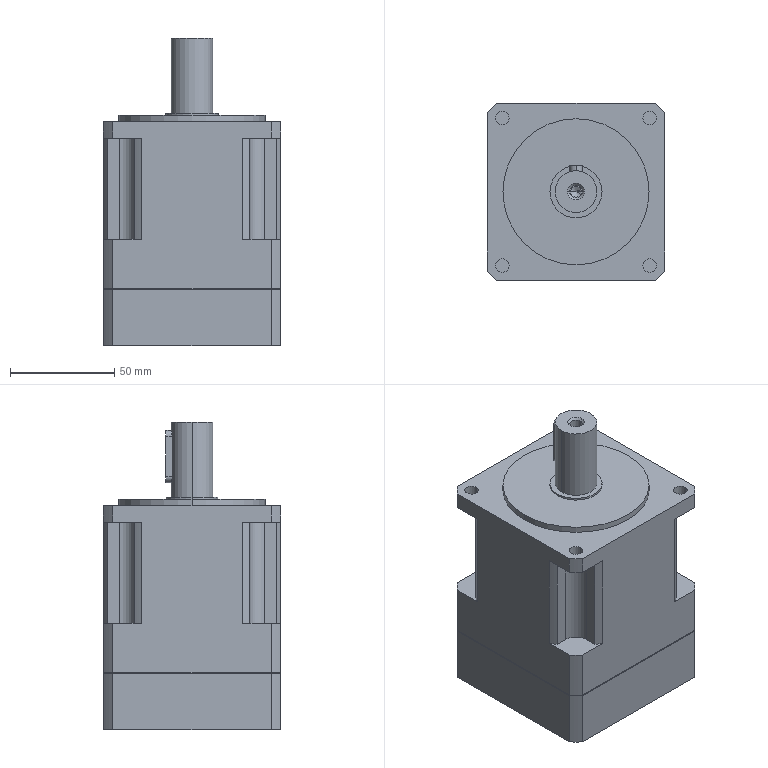Part | SolidWorks | features BaseBody 1 | 1 solid | 125 faces | box 85 x 85 x 147.5 mm | volume 726457 mm3 | cylinder 69 | plane 40 | cone 12 | spline 4 | commonest cylinder face diameters 6 x13 114 x12 5 x8 6.5 x8 98 x8 1 x4